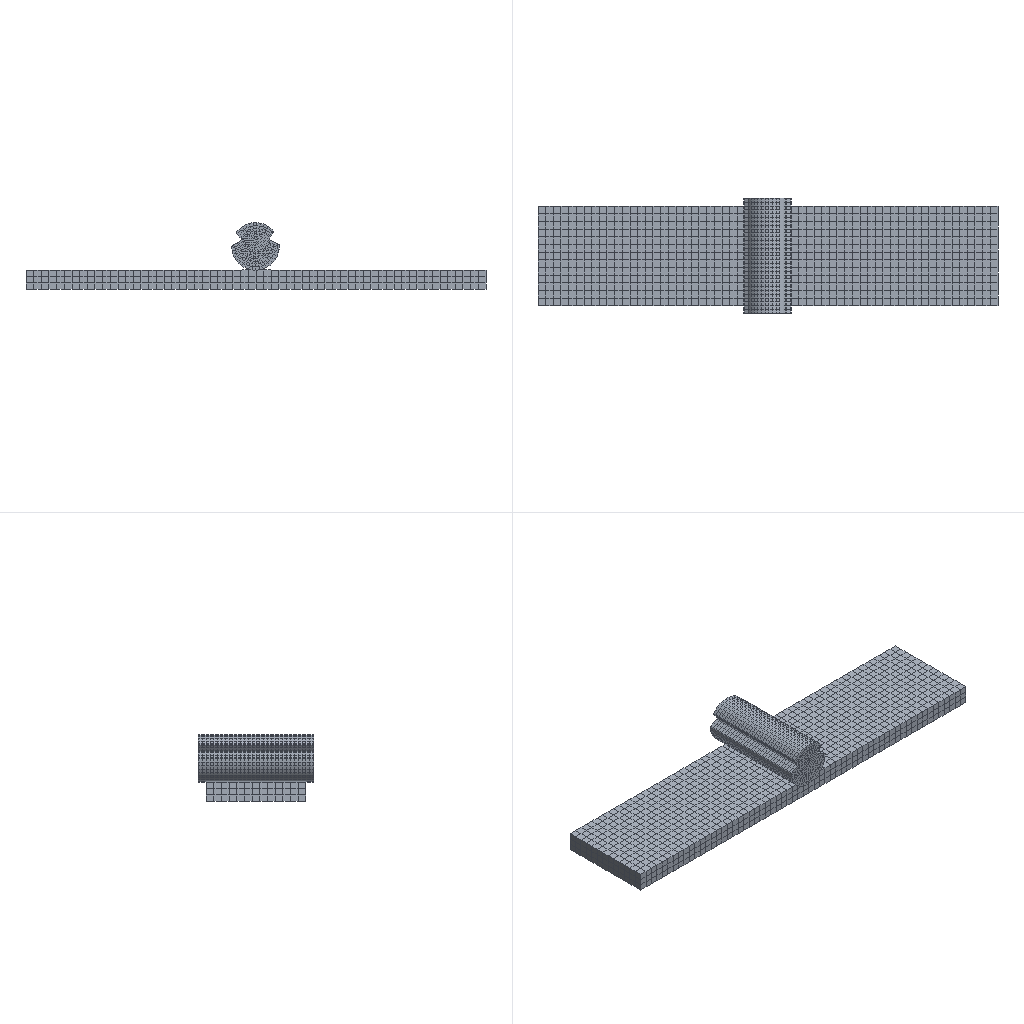Simulation study | abaqus
Set-up summary:
category,name,step,type,value,unit,region
solver,abaqus
solver,version,,,Abaqus/Standard 2020
units,not stated in the deck,,not stated
analysis,deck,,coupled thermal-electrical,coupled thermal-electrical
load_step,Step-1,Step-1,coupled thermal-electrical
load_step,requested,,,1
mesh,nodes,,,13088
mesh,elements,,,10920
element_type,DC3D8E,,solid,10920
load,load commands in deck,,count,3
bc,support commands in deck,,count,4
material,TAN,,in results
material,XIAN,,in results
check,setup vs results,,match,"per instance, exact: element labels, types and connectivity; labels of the nodes the elements use; coordinates not compared"
Abaqus input file, long lists of numbers shortened:
*Heading
** Job name: Job-1 Model name: Model-1
** Generated by: Abaqus/CAE 2020
*Preprint, echo=NO, model=NO, history=NO, contact=NO
**
** PARTS
**
*Part, name=P222
*Node
      1,         120.,         -23.,           5.
      2,         120.,         -23.,   3.333
** (3414 more lines like these left out)
*Element, type=DC3D8E
   1,   57,   58,   62,   61,    1,    2,    6,    5
   2,   58,   59,   63,   62,    2,    3,    7,    6
** (2338 more lines like these left out)
*Nset, nset=Set-2, generate
    1,  3416,     1
*Elset, elset=Set-2, generate
    1,  2340,     1
** Section: tan
*Solid Section, elset=Set-2, material=tan
,
*End Part
**
*Part, name=dao
*Node
      1,   -6.104,  0.109,           0.
      2,  -5.946,  0.3737,           0.
** (9670 more lines like these left out)
*Element, type=DC3D8E
   1,  164,  141,  127,  162,  476,  453,  439,  474
   2,  276,  162,  127,  277,  588,  474,  439,  589
** (8578 more lines like these left out)
*Nset, nset=Set-2, generate
    1,  9672,     1
*Elset, elset=Set-2, generate
    1,  8580,     1
** Section: xian
*Solid Section, elset=Set-2, material=xian
,
*End Part
**
**
** ASSEMBLY
**
*Assembly, name=Assembly
**
*Instance, name=P222-1, part=P222
*End Instance
**
*Instance, name=dao-1, part=dao
   59.767,           5.,    11.079
   59.767,           5.,    11.079, 60.767,           5.,    11.079, 90.
*End Instance
**
*Nset, nset=Set-1, instance=P222-1, generate
    1,  3416,     1
*Nset, nset=Set-1, instance=dao-1, generate
    1,  9672,     1
*Elset, elset=Set-1, instance=P222-1, generate
    1,  2340,     1
*Elset, elset=Set-1, instance=dao-1, generate
    1,  8580,     1
*Nset, nset=Set-2, instance=dao-1
    2,    3,    5,    6,   16,   17,   19,   20,   33,   34,   40,   41,  314,  315,  317,  318
  328,  329,  331,  332,  345,  346,  352,  353,  626,  627,  629,  630,  640,  641,  643,  644
** (22 more lines like these left out)
*Elset, elset=Set-2, instance=dao-1
   11,   28,   40,   89,   94,  175,  203,  273,  297,  314,  326,  375,  380,  461,  489,  559
  583,  600,  612,  661,  666,  747,  775,  845,  869,  886,  898,  947,  952, 1033, 1061, 1131
** (13 more lines like these left out)
*Nset, nset=Set-3, instance=P222-1, generate
    1,  3416,     1
*Nset, nset=Set-3, instance=dao-1, generate
   1,  312,    1
*Elset, elset=Set-3, instance=P222-1, generate
    1,  2340,     1
*Elset, elset=Set-3, instance=dao-1, generate
   1,  286,    1
*Nset, nset=Set-4, instance=dao-1, generate
   1,  312,    1
*Elset, elset=Set-4, instance=dao-1, generate
   1,  286,    1
*Elset, elset=_Surf-1_S2, internal, instance=dao-1, generate
 8295,  8580,     1
*Surface, type=ELEMENT, name=Surf-1
_Surf-1_S2, S2
*Elset, elset=_Surf-2_S3, internal, instance=P222-1
    1,    2,    3,   40,   41,   42,   79,   80,   81,  118,  119,  120,  157,  158,  159,  196
  197,  198,  235,  236,  237,  274,  275,  276,  313,  314,  315,  352,  353,  354,  391,  392
** (10 more lines like these left out)
*Elset, elset=_Surf-2_S3, internal, instance=dao-1
    8,   26,   63,   64,   86,   88,   89,   91,  101,  132,  147,  149,  157,  162,  179,  188
  190,  195,  197,  203,  204,  210,  217,  222,  294,  312,  349,  350,  372,  374,  375,  377
** (43 more lines like these left out)
*Elset, elset=_Surf-2_S5, internal, instance=P222-1
   37,   38,   39,   76,   77,   78,  115,  116,  117,  154,  155,  156,  193,  194,  195,  232
  233,  234,  271,  272,  273,  310,  311,  312,  349,  350,  351,  388,  389,  390,  427,  428
** (10 more lines like these left out)
*Elset, elset=_Surf-2_S5, internal, instance=dao-1
   28,   45,   54,   69,   93,  175,  191,  209,  215,  218,  220,  226,  230,  231,  233,  314
  331,  340,  355,  379,  461,  477,  495,  501,  504,  506,  512,  516,  517,  519,  600,  617
** (27 more lines like these left out)
*Elset, elset=_Surf-2_S1, internal, instance=P222-1, generate
 2302,  2340,     1
*Elset, elset=_Surf-2_S1, internal, instance=dao-1, generate
   1,  286,    1
*Elset, elset=_Surf-2_S4, internal, instance=P222-1, generate
    3,  2340,     3
*Elset, elset=_Surf-2_S4, internal, instance=dao-1
    9,   11,   33,   34,   40,   42,   94,  273,  295,  297,  319,  320,  326,  328,  380,  559
  581,  583,  605,  606,  612,  614,  666,  845,  867,  869,  891,  892,  898,  900,  952, 1131
** (13 more lines like these left out)
*Elset, elset=_Surf-2_S2, internal, instance=P222-1, generate
  1,  39,   1
*Elset, elset=_Surf-2_S2, internal, instance=dao-1, generate
 8295,  8580,     1
*Elset, elset=_Surf-2_S6, internal, instance=P222-1, generate
    1,  2338,     3
*Elset, elset=_Surf-2_S6, internal, instance=dao-1
   14,   24,   63,  300,  310,  349,  586,  596,  635,  872,  882,  921, 1158, 1168, 1207, 1444
 1454, 1493, 1730, 1740, 1779, 2016, 2026, 2065, 2302, 2312, 2351, 2588, 2598, 2637, 2874, 2884
** (4 more lines like these left out)
*Surface, type=ELEMENT, name=Surf-2
_Surf-2_S3, S3
_Surf-2_S5, S5
_Surf-2_S4, S4
_Surf-2_S2, S2
_Surf-2_S6, S6
_Surf-2_S1, S1
*Elset, elset=_Surf-3_S3, internal, instance=P222-1
    1,    2,    3,   40,   41,   42,   79,   80,   81,  118,  119,  120,  157,  158,  159,  196
  197,  198,  235,  236,  237,  274,  275,  276,  313,  314,  315,  352,  353,  354,  391,  392
** (10 more lines like these left out)
*Elset, elset=_Surf-3_S3, internal, instance=dao-1
    8,   26,   63,   64,   86,   88,   89,   91,  101,  132,  147,  149,  157,  162,  179,  188
  190,  195,  197,  203,  204,  210,  217,  222,  294,  312,  349,  350,  372,  374,  375,  377
** (43 more lines like these left out)
*Elset, elset=_Surf-3_S5, internal, instance=P222-1
   37,   38,   39,   76,   77,   78,  115,  116,  117,  154,  155,  156,  193,  194,  195,  232
  233,  234,  271,  272,  273,  310,  311,  312,  349,  350,  351,  388,  389,  390,  427,  428
** (10 more lines like these left out)
*Elset, elset=_Surf-3_S5, internal, instance=dao-1
   28,   45,   54,   69,   93,  175,  191,  209,  215,  218,  220,  226,  230,  231,  233,  314
  331,  340,  355,  379,  461,  477,  495,  501,  504,  506,  512,  516,  517,  519,  600,  617
** (27 more lines like these left out)
*Elset, elset=_Surf-3_S1, internal, instance=P222-1, generate
 2302,  2340,     1
*Elset, elset=_Surf-3_S1, internal, instance=dao-1, generate
   1,  286,    1
*Elset, elset=_Surf-3_S4, internal, instance=P222-1, generate
    3,  2340,     3
*Elset, elset=_Surf-3_S4, internal, instance=dao-1
    9,   11,   33,   34,   40,   42,   94,  273,  295,  297,  319,  320,  326,  328,  380,  559
  581,  583,  605,  606,  612,  614,  666,  845,  867,  869,  891,  892,  898,  900,  952, 1131
** (13 more lines like these left out)
*Elset, elset=_Surf-3_S2, internal, instance=P222-1, generate
  1,  39,   1
*Elset, elset=_Surf-3_S2, internal, instance=dao-1, generate
 8295,  8580,     1
*Elset, elset=_Surf-3_S6, internal, instance=P222-1, generate
    1,  2338,     3
*Elset, elset=_Surf-3_S6, internal, instance=dao-1
   14,   24,   63,  300,  310,  349,  586,  596,  635,  872,  882,  921, 1158, 1168, 1207, 1444
 1454, 1493, 1730, 1740, 1779, 2016, 2026, 2065, 2302, 2312, 2351, 2588, 2598, 2637, 2874, 2884
** (4 more lines like these left out)
*Surface, type=ELEMENT, name=Surf-3
_Surf-3_S3, S3
_Surf-3_S5, S5
_Surf-3_S4, S4
_Surf-3_S2, S2
_Surf-3_S6, S6
_Surf-3_S1, S1
*Elset, elset=_m_Surf-4_S3, internal, instance=dao-1
   26,   86,  101,  157,  162,  179,  188,  190,  195,  197,  204,  217,  222,  312,  372,  387
  443,  448,  465,  474,  476,  481,  483,  490,  503,  508,  598,  658,  673,  729,  734,  751
** (23 more lines like these left out)
*Elset, elset=_m_Surf-4_S4, internal, instance=dao-1, generate
   33,  8327,   286
*Elset, elset=_m_Surf-4_S5, internal, instance=dao-1
   54,  191,  215,  218,  220,  226,  340,  477,  501,  504,  506,  512,  626,  763,  787,  790
  792,  798,  912, 1049, 1073, 1076, 1078, 1084, 1198, 1335, 1359, 1362, 1364, 1370, 1484, 1621
** (10 more lines like these left out)
*Surface, type=ELEMENT, name=m_Surf-4
_m_Surf-4_S3, S3
_m_Surf-4_S4, S4
_m_Surf-4_S5, S5
*Elset, elset=_s_Surf-4_S6, internal, instance=P222-1, generate
    1,  2338,     3
*Surface, type=ELEMENT, name=s_Surf-4
_s_Surf-4_S6, S6
** Constraint: Constraint-1
*Tie, name=Constraint-1, adjust=yes
s_Surf-4, m_Surf-4
*End Assembly
**
** MATERIALS
**
*Material, name=tan
*Conductivity
3.,
*Density
 1.67e-09,
*Elastic
36500., 0.425
*Electrical Conductivity
 0.0005,
*Expansion
 3.5e-06,
*Specific Heat
 7.69e+08,
*Material, name=xian
*Conductivity
390.,
*Density
 8.9e-09,
*Elastic
110000., 0.32
*Electrical Conductivity
 0.002,
*Expansion
 1.66e-06,
*Plastic
250.,0.
*Specific Heat
 3.84e+08,
**
** PHYSICAL CONSTANTS
**
*Physical Constants, absolute zero=-273., stefan boltzmann=5.67e-08
**
** BOUNDARY CONDITIONS
**
** Name: BC-1 Type: 对称/反对称/完全固定
*Boundary
Set-2, ENCASTRE
**
** PREDEFINED FIELDS
**
** Name: Predefined Field-1   Type: Temperature
*Initial Conditions, type=TEMPERATURE
Set-1, 25.
** ----------------------------------------------------------------
**
** STEP: Step-1
**
*Step, name=Step-1, nlgeom=NO, inc=10000
*Coupled Thermal-electrical, steady state, deltmx=100000., mxdem=1.
1., 6000., 0.06, 6000.,
**
** BOUNDARY CONDITIONS
**
** Name: BC-2 Type: 电势
*Boundary
Set-4, 9, 9
**
** LOADS
**
** Name: Load-1   Type: Surface current
*Dsecurrent
Surf-1,CS,1.
**
** INTERACTIONS
**
** Interaction: Int-1
*Sradiate
Surf-2, R, 25., 0.1
** Interaction: Int-2
*Sfilm
Surf-3, F, 25., 0.2
**
** OUTPUT REQUESTS
**
*Restart, write, frequency=0
**
** FIELD OUTPUT: F-Output-1
**
*Output, field
*Node Output
CECHG, CECUR, EPOT, NT, RFL
*Element Output, directions=YES
ECD, EPG, HFL, TEMP
*Contact Output
ECD,
**
** HISTORY OUTPUT: H-Output-1
**
*Output, history, variable=PRESELECT
*End Step
Results summary:
result,step,,partial,increments=0 time=0.0/6000.0
result,analysis,,,"coupled thermal-electrical, steady state"
result,last_loadstep,,,1
result,primary field,,,"EPOT, NT11"